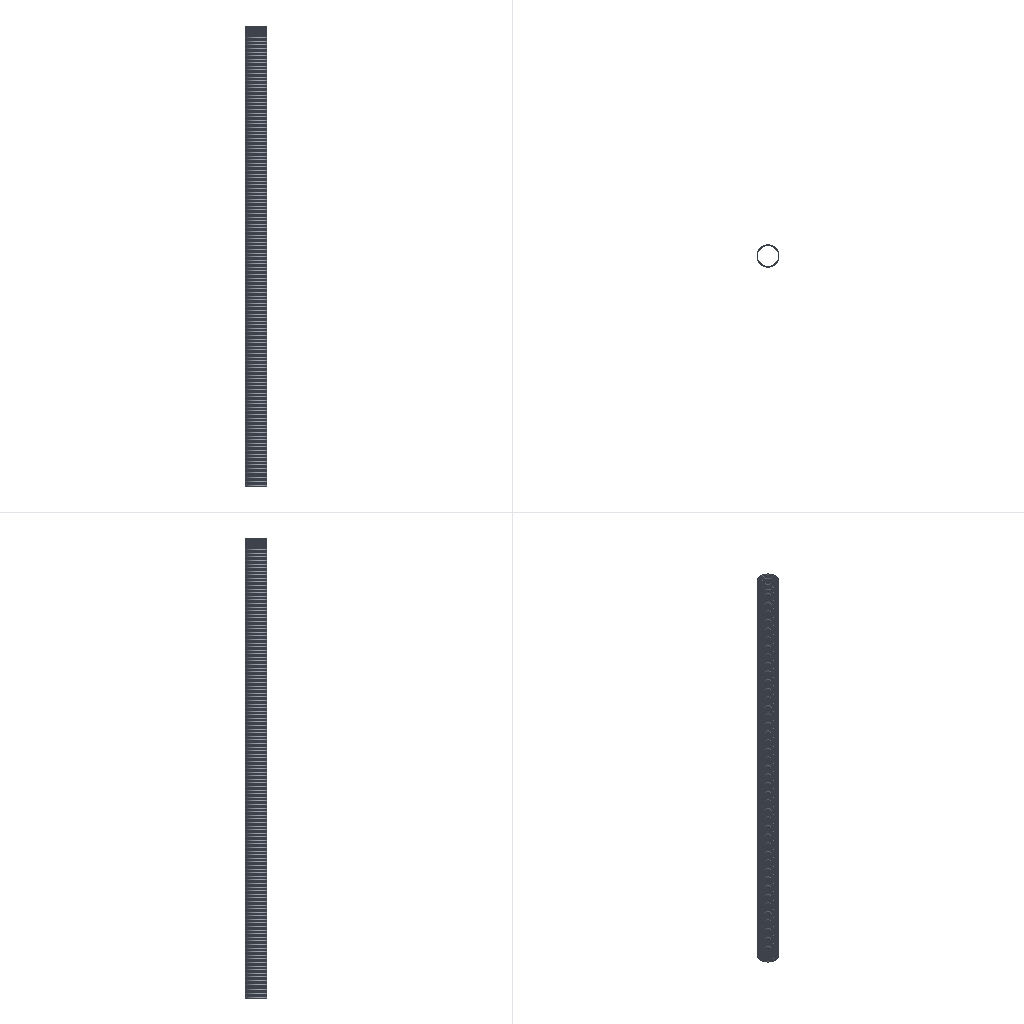Simulation study | abaqus
Set-up summary:
category,name,step,type,value,unit,region
solver,abaqus
solver,version,,,Abaqus/Explicit 3DEXPERIENCE R2017x
units,not stated in the deck,,not stated
analysis,deck,,transient,transient
load_step,Push,Push,transient
load_step,Blow,Blow,transient
load_step,requested,,,2
mesh,nodes,,,29969
mesh,elements,,,29094
element_type,S4R,,shell,16600
element_type,R3D3,,rigid,213
element_type,R3D4,,rigid,12281
load,load commands in deck,,count,4
bc,support commands in deck,,count,56
material,PET,,in results
check,setup vs results,,match,"per instance, exact: element labels, types and connectivity; labels of the nodes the elements use; coordinates of those nodes at SINGLE_PRECISION in 3 of 3 instance(s)"
Abaqus input file, long lists of numbers shortened:
*Heading
** Job name: BlowMolding Model name: Model-1_blowmolding
** Generated by: Abaqus/CAE 2017
*Preprint, echo=NO, model=NO, history=NO, contact=NO
**
** PARTS
**
*Part, name=Tube
*Node
      1,           0.,   7.8,   173.7
      2,   7.8,           0.,   173.7
** (16698 more lines like these left out)
*Element, type=S4R
   1,    1,   31, 1341,  218
   2,   31,   32, 1342, 1341
** (16598 more lines like these left out)
*Nset, nset=Bottom
    17,    18,    19,    20,    21,    27,    28,    29,    30,   796,   797,   798,   799,   800,   801,   802
   803,   804,   805,   806,   807,   808,   809,   810,   811,   812,   813,   814,   815,   816,   817,   818
** (42 more lines like these left out)
*Elset, elset=Bottom
  9076,  9077,  9078,  9079,  9080,  9081,  9082,  9083,  9084,  9085,  9086,  9087,  9088,  9089,  9090,  9091
  9092,  9093,  9094,  9095,  9096,  9097,  9098,  9099,  9100,  9101,  9102,  9103,  9104,  9105,  9106,  9107
** (36 more lines like these left out)
*Nset, nset=TopBC
    11,    12,    13,    14,    15,    22,    23,    24,    25,   643,   644,   645,   646,   647,   648,   649
   650,   651,   652,   653,   654,   655,   656,   657,   658,   659,   660,   661,   662,   663,   664,   665
** (23 more lines like these left out)
*Elset, elset=TopBC
  7101,  7102,  7103,  7104,  7105,  7106,  7107,  7108,  7109,  7110,  7111,  7112,  7113,  7114,  7115,  7116
  7117,  7118,  7119,  7120,  7121,  7122,  7123,  7124,  7125,  7126,  7127,  7128,  7129,  7130,  7131,  7132
** (17 more lines like these left out)
*Nset, nset=Set-1
     1,     2,     3,     4,     5,     6,     7,     8,     9,    10,    11,    12,    13,    14,    15,    16
    22,    23,    24,    25,    26,    31,    32,    33,    34,    35,    36,    37,    38,    39,    40,    41
** (942 more lines like these left out)
*Elset, elset=Set-1
     1,     2,     3,     4,     5,     6,     7,     8,     9,    10,    11,    12,    13,    14,    15,    16
    17,    18,    19,    20,    21,    22,    23,    24,    25,    26,    27,    28,    29,    30,    31,    32
** (936 more lines like these left out)
*Nset, nset=Set-4
     3,     4,    10,    16,    17,    18,    19,    20,    21,    27,    28,    29,    30,   125,   126,   127
   128,   129,   130,   131,   132,   133,   134,   135,   136,   137,   138,   139,   140,   141,   142,   143
** (105 more lines like these left out)
*Elset, elset=Set-4
  9076,  9077,  9078,  9079,  9080,  9081,  9082,  9083,  9084,  9085,  9086,  9087,  9088,  9089,  9090,  9091
  9092,  9093,  9094,  9095,  9096,  9097,  9098,  9099,  9100,  9101,  9102,  9103,  9104,  9105,  9106,  9107
** (98 more lines like these left out)
*Nset, nset=SymmX
    1,    4,    7,    8,    9,   10,   17,   18,   27,   28,  149,  150,  151,  152,  153,  154
  155,  156,  157,  158,  159,  160,  161,  162,  163,  164,  165,  166,  167,  168,  169,  170
** (18 more lines like these left out)
*Elset, elset=SymmX
     1,    26,    51,    76,   101,   126,   151,   176,   201,   226,   251,   276,   301,   326,   351,   376
   401,   426,   451,   476,   501,   526,   551,   576,   601,   626,   651,   676,   701,   726,   751,   776
** (38 more lines like these left out)
*Nset, nset=SymmY
    2,    3,    5,    6,   16,   19,   20,   21,   26,   29,   55,   56,   57,   58,   59,   60
   61,   62,   63,   64,   65,   66,   67,   68,   69,   70,   71,   72,   73,   74,   75,   76
** (18 more lines like these left out)
*Elset, elset=SymmY
    25,    50,    75,   100,   125,   150,   175,   200,   225,   250,   275,   300,   325,   350,   375,   400
   425,   450,   475,   500,   525,   550,   575,   600,   625,   650,   675,   700,   725,   750,   775,   800
** (38 more lines like these left out)
*Nset, nset=YSymBot
   19,   20,   21,   29,  825,  826,  827,  828,  829, 1121, 1122, 1123, 1124, 1125
*Elset, elset=YSymBot
  9220,  9221,  9222,  9223,  9224,  9225, 11845, 11846, 11847, 11848, 11849, 11850, 16195, 16196, 16197, 16198
 16199, 16200, 16595, 16596, 16597, 16598, 16599, 16600
*Nset, nset=Center
   1,   2,   5,   8,  31,  32,  33,  34,  35,  36,  37,  38,  39,  40,  41,  42
  43,  44,  45,  46,  47,  48,  49,  50,  51,  52,  53,  54, 219, 220, 221, 222
** (5 more lines like these left out)
*Elset, elset=Center
     1,     2,     3,     4,     5,     6,     7,     8,     9,    10,    11,    12,    13,    14,    15,    16
    17,    18,    19,    20,    21,    22,    23,    24,    25,  1776,  1777,  1778,  1779,  1780,  1781,  1782
** (11 more lines like these left out)
*Elset, elset=_Bottom_SNEG, internal
  9076,  9077,  9078,  9079,  9080,  9081,  9082,  9083,  9084,  9085,  9086,  9087,  9088,  9089,  9090,  9091
  9092,  9093,  9094,  9095,  9096,  9097,  9098,  9099,  9100,  9101,  9102,  9103,  9104,  9105,  9106,  9107
** (98 more lines like these left out)
*Surface, type=ELEMENT, name=Bottom
_Bottom_SNEG, SNEG
*Elset, elset=_Botout_SPOS, internal
  9076,  9077,  9078,  9079,  9080,  9081,  9082,  9083,  9084,  9085,  9086,  9087,  9088,  9089,  9090,  9091
  9092,  9093,  9094,  9095,  9096,  9097,  9098,  9099,  9100,  9101,  9102,  9103,  9104,  9105,  9106,  9107
** (98 more lines like these left out)
*Surface, type=ELEMENT, name=Botout
_Botout_SPOS, SPOS
*Elset, elset=_Interior_SNEG, internal
     1,     2,     3,     4,     5,     6,     7,     8,     9,    10,    11,    12,    13,    14,    15,    16
    17,    18,    19,    20,    21,    22,    23,    24,    25,    26,    27,    28,    29,    30,    31,    32
** (886 more lines like these left out)
*Surface, type=ELEMENT, name=Interior
_Interior_SNEG, SNEG
*Elset, elset=_Exterior_SPOS, internal
     1,     2,     3,     4,     5,     6,     7,     8,     9,    10,    11,    12,    13,    14,    15,    16
    17,    18,    19,    20,    21,    22,    23,    24,    25,    26,    27,    28,    29,    30,    31,    32
** (917 more lines like these left out)
*Surface, type=ELEMENT, name=Exterior
_Exterior_SPOS, SPOS
** Section: Tube
*Shell Section, elset=Set-1, material=PET, controls=EC-1
2.5, 5
** Section: Tube
*Shell Section, elset=Set-4, material=PET, controls=EC-1
2.5, 5
*End Part
**
*Part, name=XNeg
*Node
     58,  -5.657,  -5.657,    321.57
     59,  -7.391,  -3.061,    321.57
** (6575 more lines like these left out)
*Element, type=R3D4
1,  1,  2, 50, 63
2, 63, 50, 51, 62
** (6078 more lines like these left out)
*Element, type=R3D3
2189, 2789, 2722, 2717
2190, 2770, 2776, 2768
** (112 more lines like these left out)
*Node
   6578,  -2.46801937e-05,  6.48498535e-05,    321.57
*Nset, nset=XNeg-RefPt_, internal
6578,
*Nset, nset=Set-1-RP-XNeg
 6578,
*Elset, elset=_Cont_SNEG, internal, generate
    1,  6194,     1
*Surface, type=ELEMENT, name=Cont
_Cont_SNEG, SNEG
*Elset, elset=XNeg, generate
    1,  6194,     1
*End Part
**
*Part, name=XPos
*Node
     38,  -5.31366641e-05,  -44.803,   34.21
     41,  3.01543005e-05,  -44.983,   26.722
** (6688 more lines like these left out)
*Element, type=R3D4
1,  1,  2, 54, 67
2, 67, 54, 55, 66
** (6199 more lines like these left out)
*Element, type=R3D3
2593, 3074, 3060, 3056
2594, 3011, 3009, 3010
** (97 more lines like these left out)
*Node
   6691,  -2.46801937e-05,  6.48498535e-05,    321.57
*Nset, nset=XPos-RefPt_, internal
6691,
*Nset, nset=Set-1-RP-XPos
 6691,
*Elset, elset=_Cont_SNEG, internal, generate
    1,  6300,     1
*Surface, type=ELEMENT, name=Cont
_Cont_SNEG, SNEG
*Elset, elset=XPos, generate
    1,  6300,     1
*End Part
**
**
** ASSEMBLY
**
*Assembly, name=Assembly
**
*Instance, name=XNeg-1, part=XNeg
         -8.,           0.,           0.
*End Instance
**
*Instance, name=XPos-1, part=XPos
          8.,           0.,           0.
*End Instance
**
*Instance, name=Tube-1, part=Tube
          0.,           0.,    -11.43
*End Instance
**
*Node
      1,           0.,  -4.77612233e-16,    321.57
*Nset, nset=Set-1_RP-Fluid
 1,
*Nset, nset=_PickedSet10, internal, instance=Tube-1
     3,     4,    10,    16,    17,    18,    19,    20,    21,    27,    28,    29,    30,   125,   126,   127
   128,   129,   130,   131,   132,   133,   134,   135,   136,   137,   138,   139,   140,   141,   142,   143
** (105 more lines like these left out)
*Elset, elset=_PickedSet10, internal, instance=Tube-1
  9076,  9077,  9078,  9079,  9080,  9081,  9082,  9083,  9084,  9085,  9086,  9087,  9088,  9089,  9090,  9091
  9092,  9093,  9094,  9095,  9096,  9097,  9098,  9099,  9100,  9101,  9102,  9103,  9104,  9105,  9106,  9107
** (98 more lines like these left out)
*Rigid Body, ref node=XNeg-1.XNeg-RefPt_, elset=XNeg-1.XNeg
*Rigid Body, ref node=XPos-1.XPos-RefPt_, elset=XPos-1.XPos
*End Assembly
**
** ELEMENT CONTROLS
**
*Section Controls, name=EC-1, hourglass=ENHANCED, second order accuracy=YES
1., 1., 1.
*Amplitude, name=Amp-1, time=TOTAL TIME
             0.,              0.,            0.05,              0.,             0.2,              1.,              1.,              1.
**
** MATERIALS
**
*Material, name=PET
*Density
 9.4e-10,
*Elastic
10., 0.3
*Plastic
 2.,  0.
 5., 0.5
20.,  1.
**
** INTERACTION PROPERTIES
**
*Fluid Behavior, name=FCavity
*Molecular Weight
6.2e-05
*Capacity, type=TABULAR
 2.811e+07,
*Fluid Exchange Property, name=FExchange, type=MASS FLUX
 -1e-07,
*Surface Interaction, name=Friction
*Friction
 0.4,
**
** PHYSICAL CONSTANTS
**
*Physical Constants, absolute zero=-273.15, universal gas=8314.34
**
** BOUNDARY CONDITIONS
**
** Name: BC-4-SET-1 Type: Velocity/Angular velocity
*Boundary, type=VELOCITY
Tube-1.Set-1, 3, 3
** Name: BC-SYMMX Type: Velocity/Angular velocity
*Boundary, type=VELOCITY
Tube-1.SymmX, 1, 1
Tube-1.SymmX, 5, 5
Tube-1.SymmX, 6, 6
** Name: BC-SYMMY Type: Velocity/Angular velocity
*Boundary, type=VELOCITY
Tube-1.SymmY, 2, 2
Tube-1.SymmY, 4, 4
Tube-1.SymmY, 6, 6
** Name: TOP-BC Type: Displacement/Rotation
*Boundary
Tube-1.TopBC, 1, 1
Tube-1.TopBC, 2, 2
Tube-1.TopBC, 4, 4
Tube-1.TopBC, 5, 5
Tube-1.TopBC, 6, 6
** Name: Xneg Type: Displacement/Rotation
*Boundary
XPos-1.Set-1-RP-XPos, 1, 1
XPos-1.Set-1-RP-XPos, 2, 2
XPos-1.Set-1-RP-XPos, 3, 3
XPos-1.Set-1-RP-XPos, 4, 4
XPos-1.Set-1-RP-XPos, 5, 5
XPos-1.Set-1-RP-XPos, 6, 6
** Name: Xpos Type: Displacement/Rotation
*Boundary
XPos-1.Set-1-RP-XPos, 1, 1
XPos-1.Set-1-RP-XPos, 2, 2
XPos-1.Set-1-RP-XPos, 3, 3
XPos-1.Set-1-RP-XPos, 4, 4
XPos-1.Set-1-RP-XPos, 5, 5
XPos-1.Set-1-RP-XPos, 6, 6
**
** INTERACTIONS
**
** Interaction: FluidCavity
*Fluid Cavity, name=FluidCavity, behavior=FCavity, refnode=Set-1_RP-Fluid, surface=Tube-1.Interior
** Interaction: FluidExchange
*Fluid Exchange, name=FluidExchange, property=FExchange, effective area=500.
Set-1_RP-Fluid
** Interaction: friction
*Contact, op=NEW
*Contact Inclusions, ALL EXTERIOR
*Contact Exclusions
Tube-1.Exterior , XNeg-1.Cont
Tube-1.Exterior , XPos-1.Cont
Tube-1.Bottom ,
Tube-1.Botout , XNeg-1.Cont
Tube-1.Botout , XPos-1.Cont
*Contact Property Assignment
 ,  , Friction
** ----------------------------------------------------------------
**
** STEP: Push
**
*Step, name=Push, nlgeom=YES
*Dynamic, Explicit
, 0.14
*Bulk Viscosity
0.06, 1.2
** Mass Scaling: Semi-Automatic
**               Whole Model
*Variable Mass Scaling, dt=4e-06, type=below min, frequency=1
**
** BOUNDARY CONDITIONS
**
** Name: Xneg Type: Displacement/Rotation
*Boundary, amplitude=Amp-1
XPos-1.Set-1-RP-XPos, 1, 1, 8.
XPos-1.Set-1-RP-XPos, 2, 2
XPos-1.Set-1-RP-XPos, 3, 3
XPos-1.Set-1-RP-XPos, 4, 4
XPos-1.Set-1-RP-XPos, 5, 5
XPos-1.Set-1-RP-XPos, 6, 6
** Name: Xpos Type: Displacement/Rotation
*Boundary, amplitude=Amp-1
XPos-1.Set-1-RP-XPos, 1, 1, -8.
XPos-1.Set-1-RP-XPos, 2, 2
XPos-1.Set-1-RP-XPos, 3, 3
XPos-1.Set-1-RP-XPos, 4, 4
XPos-1.Set-1-RP-XPos, 5, 5
XPos-1.Set-1-RP-XPos, 6, 6
*Fluid Exchange Activation
FluidExchange
**
** OUTPUT REQUESTS
**
*Restart, write, number interval=1, time marks=NO
**
** FIELD OUTPUT: F-Output-2
**
*Output, field
*Element Output, directions=YES
STH,
**
** FIELD OUTPUT: F-Output-1
**
*Output, field, variable=PRESELECT
**
** HISTORY OUTPUT: H-Output-1
**
*Output, history, variable=PRESELECT
*End Step
** ----------------------------------------------------------------
**
** STEP: Blow
**
*Step, name=Blow, nlgeom=YES
*Dynamic, Explicit
, 0.5
*Bulk Viscosity
0.06, 1.2
**
** BOUNDARY CONDITIONS
**
** Name: BC-4-SET-1 Type: Velocity/Angular velocity
*Boundary, op=NEW
** Name: BC-SYMMX Type: Velocity/Angular velocity
*Boundary, op=NEW
** Name: BC-SYMMY Type: Velocity/Angular velocity
*Boundary, op=NEW
** Name: BC-bot Type: Velocity/Angular velocity
*Boundary, op=NEW, type=VELOCITY
Tube-1.YSymBot, 2, 2
Tube-1.YSymBot, 4, 4
Tube-1.YSymBot, 6, 6
** Name: TOP-BC Type: Displacement/Rotation
*Boundary, op=NEW
Tube-1.TopBC, 1, 1
Tube-1.TopBC, 2, 2
Tube-1.TopBC, 4, 4
Tube-1.TopBC, 5, 5
Tube-1.TopBC, 6, 6
** Name: Xneg Type: Displacement/Rotation
*Boundary, op=NEW, amplitude=Amp-1
XPos-1.Set-1-RP-XPos, 1, 1, 8.
XPos-1.Set-1-RP-XPos, 2, 2
XPos-1.Set-1-RP-XPos, 3, 3
XPos-1.Set-1-RP-XPos, 4, 4
XPos-1.Set-1-RP-XPos, 5, 5
XPos-1.Set-1-RP-XPos, 6, 6
** Name: Xpos Type: Displacement/Rotation
*Boundary, op=NEW, amplitude=Amp-1
XPos-1.Set-1-RP-XPos, 1, 1, -8.
XPos-1.Set-1-RP-XPos, 2, 2
XPos-1.Set-1-RP-XPos, 3, 3
XPos-1.Set-1-RP-XPos, 4, 4
XPos-1.Set-1-RP-XPos, 5, 5
XPos-1.Set-1-RP-XPos, 6, 6
**
** OUTPUT REQUESTS
**
*Restart, write, number interval=1, time marks=NO
**
** FIELD OUTPUT: F-Output-2
**
*Output, field
*Element Output, directions=YES
STH,
**
** FIELD OUTPUT: F-Output-1
**
*Output, field, variable=PRESELECT
**
** HISTORY OUTPUT: H-Output-1
**
*Output, history, variable=PRESELECT
*End Step
Results summary:
result,step,Push,completed,increments=35397 time=0.14/0.14
result,step,Blow,completed,increments=130818 time=0.5/0.5
result,analysis,,,transient
result,last_loadstep,,,2
result,primary field,,,"U, UR"
result,reaction total,,FX,-16.912,model units
result,reaction total,,FY,2.99,model units
result,reaction total,,FZ,-1064.009,model units